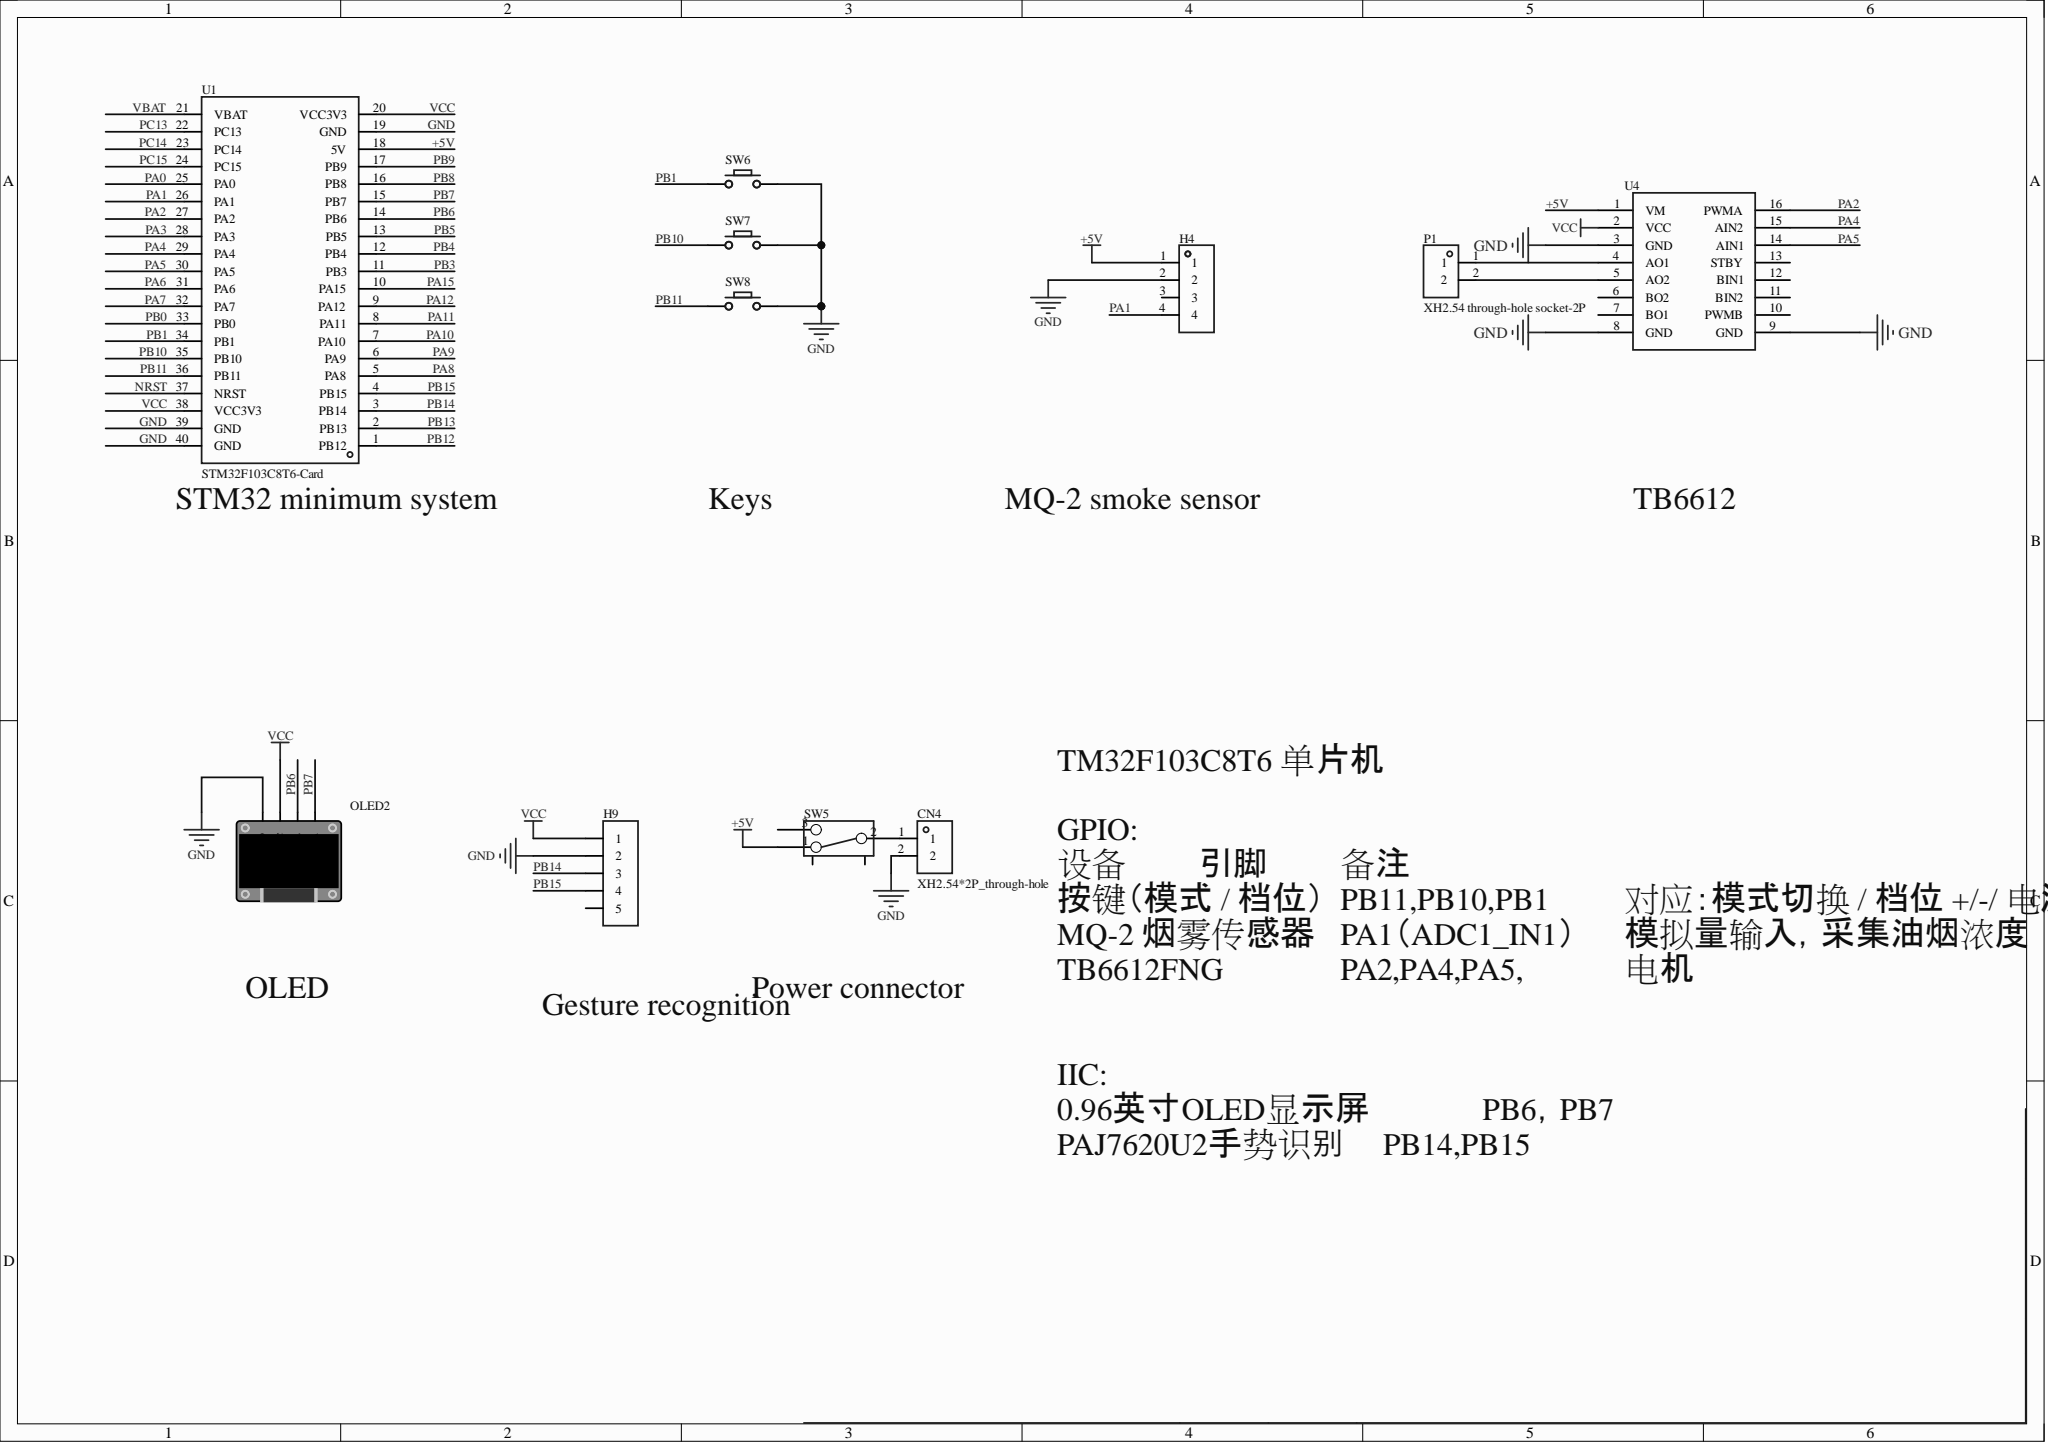Circuit board | Altium Designer | 11 parts | 17 nets
Bill of materials:
Comment,Description,Designator,Footprint,LibRef,Quantity
"XH2.54*2P_through-hole","","CN4","CONN-TH_2P-P2.50-XH2.54-2P","XH2.54*2P_直插","1"
"","","H4","HDR-TH_4P-P2.54-V-F","HDR-F_2.54_1x4P","1"
"","","H9","HDR-TH_5P-P2.54-V-F","HDR-F_2.54_1x5P","1"
"","","OLED2","0.96OLED_4P","0.96OLED模块_4P","1"
"XH2.54 through-hole socket-2P","","P1","CONN-TH_XH2.54-2P","XH2.54直插座-2P","1"
"","","SW5","拨动开关","拨动开关_正","1"
"","","SW6, SW7, SW8","Key_TH_3.5x6x4.3","Key_TH_3.5x6x4.3","3"
"STM32F103C8T6-Card","","U1","CONN-TH_L53.3-W22.9_STM32F103C8T6-CARD","STM32F103C8T6-Card","1"
"","","U4","tb6612","tb6612","1"
Netlist (Protel format):
[
CN4
CONN-TH_2P-P2.50-XH2.54-2P
XH2.54*2P_through-hole



]
[
H4
HDR-TH_4P-P2.54-V-F




]
[
H9
HDR-TH_5P-P2.54-V-F




]
[
OLED2
0.96OLED_4P




]
[
P1
CONN-TH_XH2.54-2P
XH2.54 through-hole socket-2P



]
[
SW5
拨动开关




]
[
SW6
Key_TH_3.5x6x4.3




]
[
SW7
Key_TH_3.5x6x4.3




]
[
SW8
Key_TH_3.5x6x4.3




]
[
U1
CONN-TH_L53.3-W22.9_STM32F103C8T6-CARD
STM32F103C8T6-Card



]
[
U4
tb6612




]
(
VCC
H9-1
OLED2-2
U1-20
U1-38
U4-2
)
(
PB15
H9-4
U1-4
)
(
PB14
H9-3
U1-3
)
(
PB11
SW8-A
U1-36
)
(
PB10
SW7-A
U1-35
)
(
PB7
OLED2-4
U1-15
)
(
PB6
OLED2-3
U1-14
)
(
PB1
SW6-A
U1-34
)
(
PA5
U1-30
U4-14
)
(
PA4
U1-29
U4-15
)
(
PA2
U1-27
U4-16
)
(
PA1
H4-4
U1-26
)
(
NetP1_2
P1-2
U4-5
)
(
NetP1_1
P1-1
U4-4
)
(
NetCN4_1
CN4-1
SW5-2
)
(
GND
CN4-2
H4-2
H9-2
OLED2-1
SW6-B
SW7-B
SW8-B
U1-19
U1-39
U1-40
U4-3
U4-8
U4-9
)
(
+5V
H4-1
SW5-1
U1-18
U4-1
)